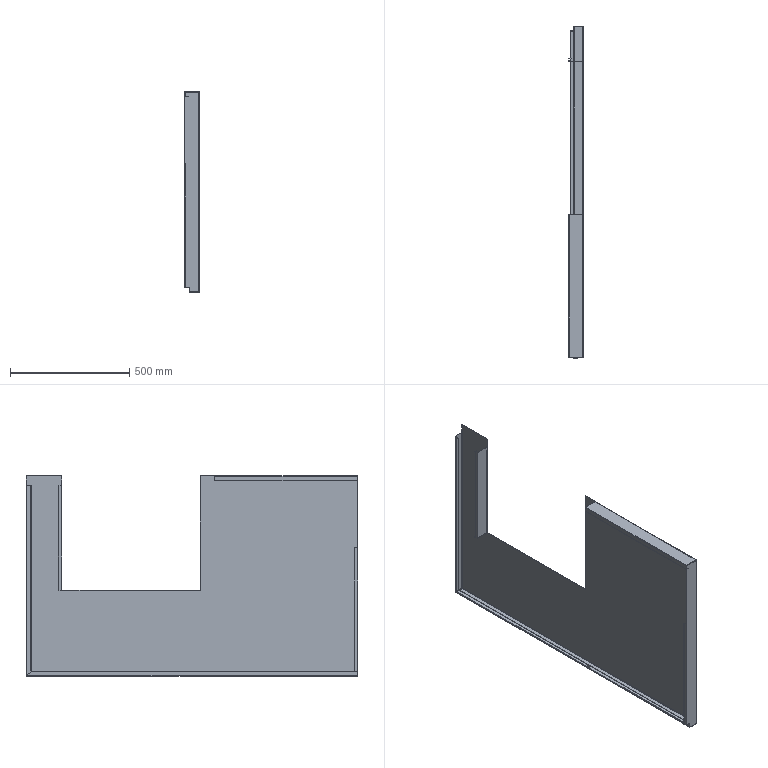Part | SolidWorks | features EdgeFlange 6, ICE 2, FlatPattern 1, SMBaseFlange 1, SheetMetal 1 | 1 solid | 142 faces | box 60 x 1390 x 840 mm | volume 1426694 mm3 | plane 107 | cylinder 29 | spline 6 | commonest cylinder face diameters 0.9 x15 3.3 x14